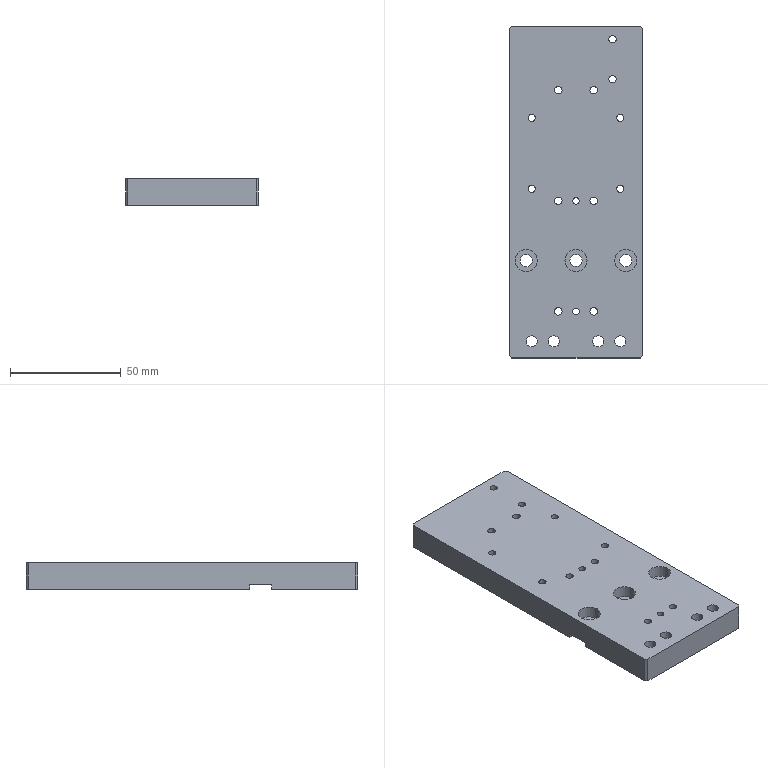Part | SolidWorks | features HoleWzd 8, ICE 2, Chamfer 1, Extrusion 1, LPattern 1 | 1 solid | 83 faces | box 60 x 150 x 12 mm | volume 102302 mm3 | cylinder 60 | plane 23 | commonest cylinder face diameters 3.3 x12 3.4 x12 6.5 x12 5 x8 5.5 x6 10 x6